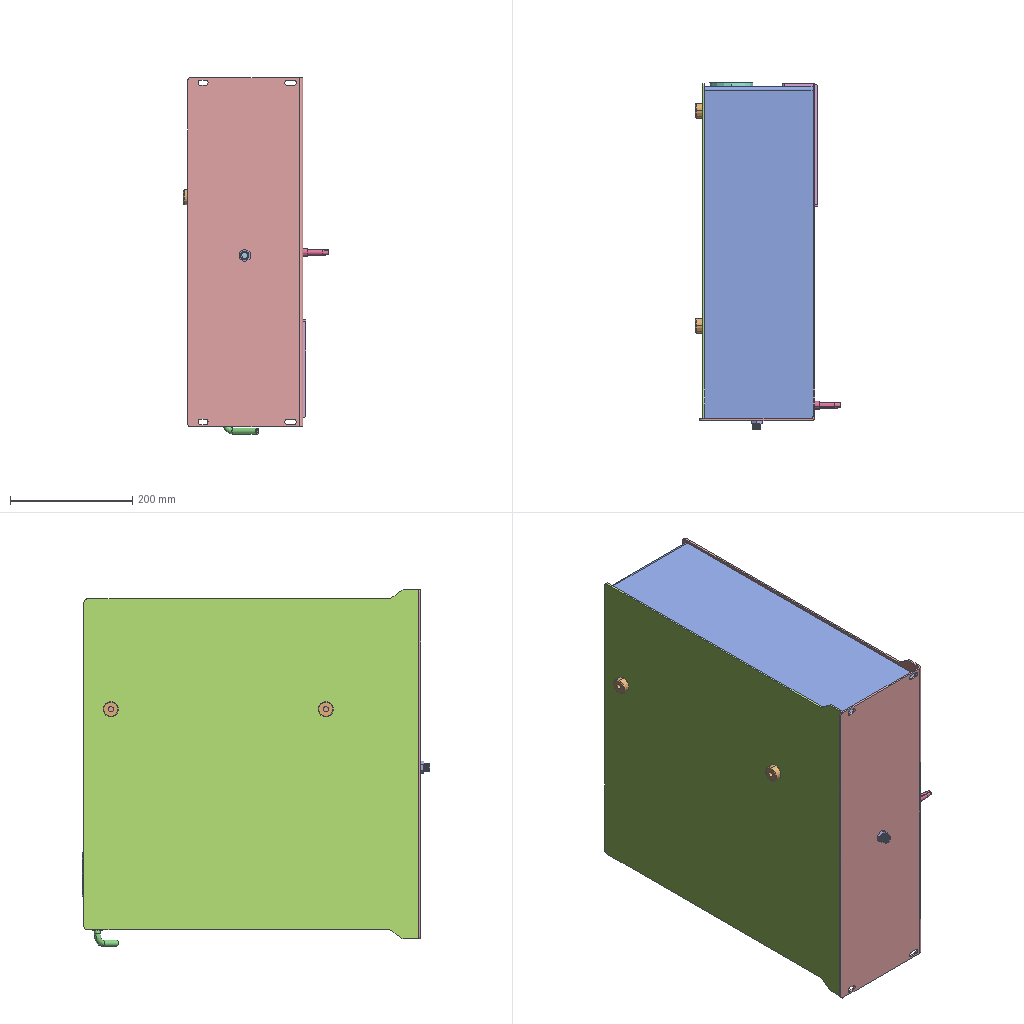Assembly | SolidWorks | 10 different items | 11 placed | box 237 x 568 x 582 mm
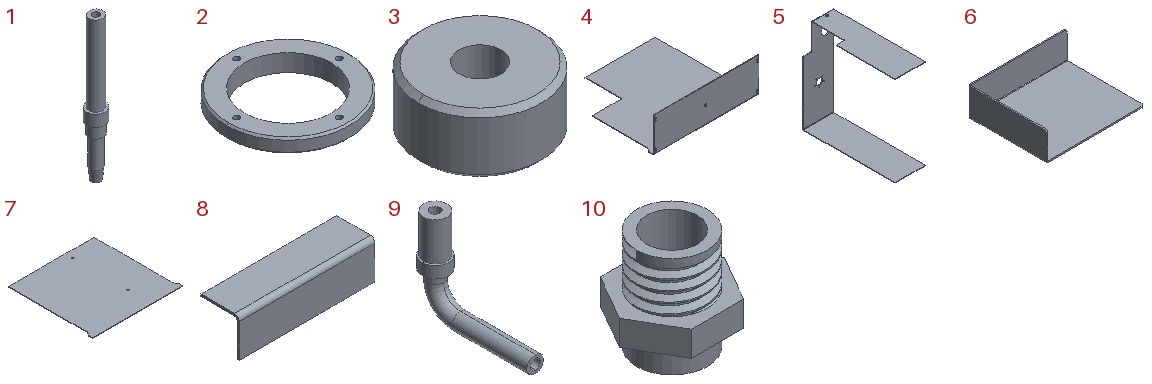Parts list (item | quantity | size | volume | features):
1 | x1 | 16 x 16 x 125 mm | 10323 mm3 | features ICE 3, Chamfer 1, Extrusion 1
2 | x1 | 71 x 71 x 10 mm | 15956 mm3 | features ICE 2, Chamfer 1, Extrusion 1, HoleWzd 1
3 | x2 | 25 x 25 x 12 mm | 5133 mm3 | features Chamfer 1, Extrusion 1, HoleWzd 1
4 | x1 | 570 x 550 x 188 mm | 1109133 mm3 | features Fillet 3, ICE 2, FlatPattern 1, SMBaseFlange 1, SheetMetal 1
5 | x1 | 177 x 542 x 530 mm | 789505 mm3 | features ICE 3, Fillet 2, FlatPattern 1, HoleWzd 1, SMBaseFlange 1, SheetMetal 1
6 | x1 | 200 x 160 x 58 mm | 153068 mm3 | features EdgeFlange 1, Fillet 1, FlatPattern 1, SMBaseFlange 1, SheetMetal 1
7 | x1 | 570 x 547 x 3 mm | 888967 mm3 | features Fillet 2, FlatPattern 1, SMBaseFlange 1, SheetMetal 1
8 | x1 | 177 x 50 x 50 mm | 50481 mm3 | features FlatPattern 1, SMBaseFlange 1, SheetMetal 1
9 | x1 | 16 x 68 x 55 mm | 7797 mm3 | features ICE 2, Sweep 1
10 | x1 | 20.785 x 18 x 20 mm | 1890 mm3 | features ICE 2, Extrusion 1, SweepThread 1
Mates (type | each side: item.copy, entity, surface, feature):
Coincident | 4.1 face plane Base-Flange1 | 5.1 face plane Base-Flange1 | 2 times
DistanceDim | 5.1 face plane Base-Flange1 | 4.1 face plane Base-Flange1
Coincident | 5.1 face plane Base-Flange1 | 7.1 face plane Base-Flange1
Coincident | 4.1 face plane Base-Flange1 | 7.1 face plane Base-Flange1 | 2 times
Coincident | 5.1 face plane Cut-Extrude1 | 6.1 face plane Base-Flange1
Coincident | 4.1 face plane Cut-Extrude1 | 6.1 face plane Edge-Flange1 | 2 times
Concentric | 5.1 face cylinder Cut-Extrude3 | 2.1 face cylinder Cut-Extrude2
Coincident | 5.1 face plane Base-Flange1 | 2.1 face plane Cut-Extrude2
Parallel | 2.1 plane | assembly plane
Coincident | 7.1 face plane Base-Flange1 | 3.1 face plane Boss-Extrude1
Concentric | 7.1 face cylinder Base-Flange1 | 3.1 face cylinder Boss-Extrude1
Coincident | 7.1 face plane Base-Flange1 | 3.2 face plane Boss-Extrude1
Concentric | 7.1 face cylinder Base-Flange1 | 3.2 face cylinder Boss-Extrude1
Coincident | 4.1 face plane Base-Flange1 | 10.1 face plane Cut-Extrude2
Concentric | 4.1 face cylinder Cut-Extrude2 | 10.1 face cylinder Boss-Extrude1
Parallel | 4.1 face plane Base-Flange1 | 10.1 face plane Boss-Extrude1
Concentric | 5.1 face cylinder Cut-Extrude2 | 9.1 face cylinder Boss-Extrude1
Coincident | 5.1 face plane Base-Flange1 | 9.1 face plane Boss-Extrude2
PlanarAngleDim | 9.1 plane | assembly plane
Concentric | 4.1 face cylinder Cut-Extrude1 | 1.1 face cylinder Boss-Extrude2
Coincident | 4.1 face plane Base-Flange1 | 1.1 face plane Boss-Extrude3
Coincident | 4.1 face plane Base-Flange1 | 8.1 face plane Base-Flange1
DistanceDim | 4.1 face plane Cut-Extrude1 | 8.1 face plane Base-Flange1
DistanceDim | 4.1 face plane Base-Flange1 | 8.1 face plane Base-Flange1